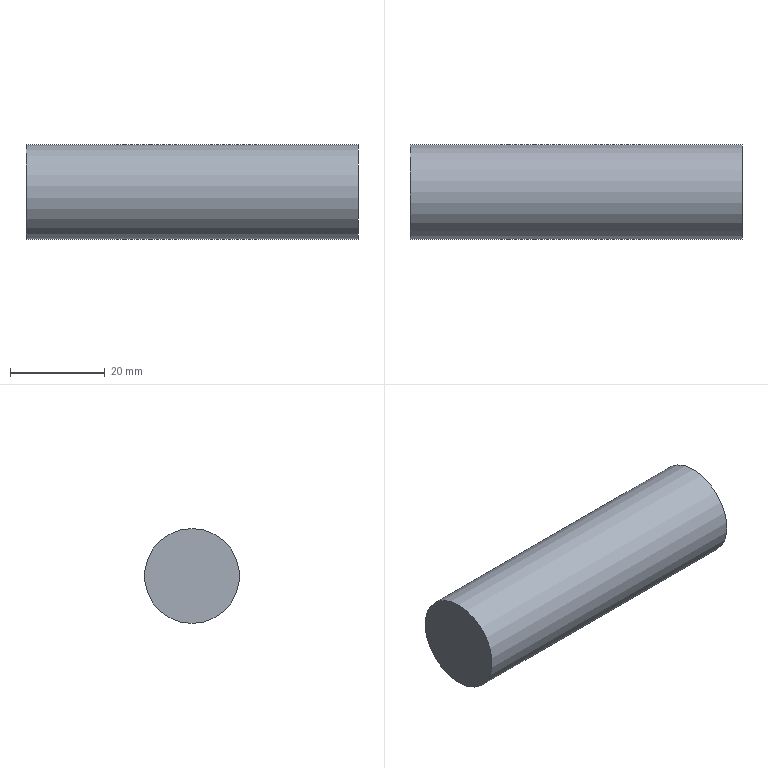Part | NX | features solid 2 | 1 solid | 3 faces | box 70 x 20 x 20 mm | volume 21991 mm3 | plane 2 | cylinder 1 | commonest cylinder face diameters 20 x1
STEP:
#1=CARTESIAN_POINT('',(15.,-180.,-459.4));
#2=VERTEX_POINT('',#1);
#3=CARTESIAN_POINT('',(15.,-180.,-449.4));
#4=DIRECTION('',(1.,0.,0.));
#5=DIRECTION('',(0.,0.,-1.));
#6=AXIS2_PLACEMENT_3D('',#3,#4,#5);
#7=CIRCLE('',#6,10.);
#8=EDGE_CURVE('',#2,#2,#7,.F.);
#9=ORIENTED_EDGE('',*,*,#8,.T.);
#10=EDGE_LOOP('',(#9));
#11=FACE_BOUND('',#10,.T.);
#12=CARTESIAN_POINT('',(-55.,-180.,-439.4));
#13=VERTEX_POINT('',#12);
#14=CARTESIAN_POINT('',(-55.,-180.,-449.4));
#15=DIRECTION('',(-1.,0.,0.));
#16=DIRECTION('',(0.,0.,1.));
#17=AXIS2_PLACEMENT_3D('',#14,#15,#16);
#18=CIRCLE('',#17,10.);
#19=EDGE_CURVE('',#13,#13,#18,.T.);
#20=ORIENTED_EDGE('',*,*,#19,.F.);
#21=EDGE_LOOP('',(#20));
#22=FACE_BOUND('',#21,.T.);
#23=CARTESIAN_POINT('',(46.,-180.,-449.4));
#24=DIRECTION('',(-1.,0.,0.));
#25=DIRECTION('',(0.,1.,0.));
#26=AXIS2_PLACEMENT_3D('',#23,#24,#25);
#27=CYLINDRICAL_SURFACE('',#26,10.);
#28=ADVANCED_FACE('',(#11,#22),#27,.T.);
#29=ORIENTED_EDGE('',*,*,#8,.F.);
#30=EDGE_LOOP('',(#29));
#31=FACE_BOUND('',#30,.T.);
#32=CARTESIAN_POINT('',(15.,-180.,-449.4));
#33=DIRECTION('',(1.,0.,0.));
#34=DIRECTION('',(0.,0.,1.));
#35=AXIS2_PLACEMENT_3D('',#32,#33,#34);
#36=PLANE('',#35);
#37=ADVANCED_FACE('',(#31),#36,.T.);
#38=ORIENTED_EDGE('',*,*,#19,.T.);
#39=EDGE_LOOP('',(#38));
#40=FACE_BOUND('',#39,.T.);
#41=CARTESIAN_POINT('',(-55.,-180.,-449.4));
#42=DIRECTION('',(1.,0.,0.));
#43=DIRECTION('',(0.,0.,1.));
#44=AXIS2_PLACEMENT_3D('',#41,#42,#43);
#45=PLANE('',#44);
#46=ADVANCED_FACE('',(#40),#45,.F.);
#47=CLOSED_SHELL('',(#28,#37,#46));
#48=MANIFOLD_SOLID_BREP('',#47);
#49=(LENGTH_UNIT()NAMED_UNIT(*)SI_UNIT(.MILLI.,.METRE.));
#50=UNCERTAINTY_MEASURE_WITH_UNIT(LENGTH_MEASURE(0.00001),#49,'','');
#51=(NAMED_UNIT(*)PLANE_ANGLE_UNIT()SI_UNIT($,.RADIAN.));
#52=(NAMED_UNIT(*)SI_UNIT($,.STERADIAN.)SOLID_ANGLE_UNIT());
#53=(GEOMETRIC_REPRESENTATION_CONTEXT(3)GLOBAL_UNCERTAINTY_ASSIGNED_CONTEXT((#50))GLOBAL_UNIT_ASSIGNED_CONTEXT((#49,#51,#52))REPRESENTATION_CONTEXT('',''));
#54=ADVANCED_BREP_SHAPE_REPRESENTATION('',(#48),#53);